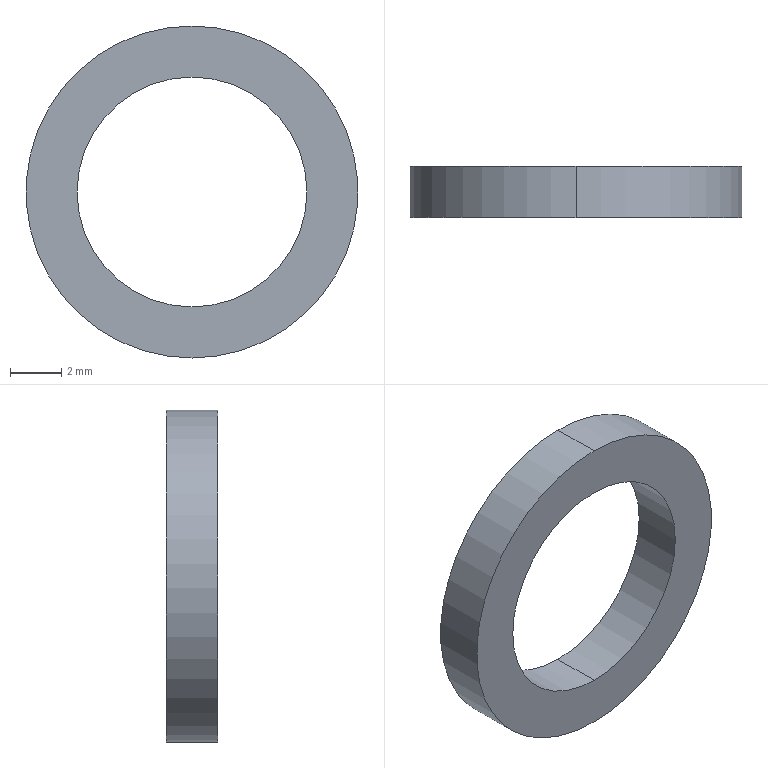Part | NX | features BREP 1 | 1 solid | 6 faces | box 13 x 2 x 13 mm | volume 138.23 mm3 | cylinder 4 | plane 2 | commonest cylinder face diameters 9 x2 13 x2
STEP:
#1=CARTESIAN_POINT('',(0.,2.,-4.5));
#2=VERTEX_POINT('',#1);
#3=CARTESIAN_POINT('',(0.,2.,4.5));
#4=VERTEX_POINT('',#3);
#5=CARTESIAN_POINT('',(0.,2.,0.));
#6=DIRECTION('',(0.,1.,0.));
#7=DIRECTION('',(0.,0.,1.));
#8=AXIS2_PLACEMENT_3D('',#5,#6,#7);
#9=CIRCLE('',#8,4.5);
#10=EDGE_CURVE('',#2,#4,#9,.T.);
#11=ORIENTED_EDGE('',*,*,#10,.T.);
#12=CARTESIAN_POINT('',(0.,0.,4.5));
#13=VERTEX_POINT('',#12);
#14=CARTESIAN_POINT('',(0.,2.,4.5));
#15=DIRECTION('',(0.,-1.,0.));
#16=VECTOR('',#15,1000.);
#17=LINE('',#14,#16);
#18=EDGE_CURVE('',#13,#4,#17,.F.);
#19=ORIENTED_EDGE('',*,*,#18,.F.);
#20=CARTESIAN_POINT('',(0.,0.,-4.5));
#21=VERTEX_POINT('',#20);
#22=CARTESIAN_POINT('',(0.,0.,0.));
#23=DIRECTION('',(0.,1.,0.));
#24=DIRECTION('',(0.,0.,1.));
#25=AXIS2_PLACEMENT_3D('',#22,#23,#24);
#26=CIRCLE('',#25,4.5);
#27=EDGE_CURVE('',#21,#13,#26,.T.);
#28=ORIENTED_EDGE('',*,*,#27,.F.);
#29=CARTESIAN_POINT('',(0.,2.,-4.5));
#30=DIRECTION('',(0.,-1.,0.));
#31=VECTOR('',#30,1000.);
#32=LINE('',#29,#31);
#33=EDGE_CURVE('',#21,#2,#32,.F.);
#34=ORIENTED_EDGE('',*,*,#33,.T.);
#35=EDGE_LOOP('',(#11,#19,#28,#34));
#36=FACE_BOUND('',#35,.T.);
#37=CARTESIAN_POINT('',(0.,2.,0.));
#38=DIRECTION('',(0.,-1.,0.));
#39=DIRECTION('',(0.,0.,1.));
#40=AXIS2_PLACEMENT_3D('',#37,#38,#39);
#41=CYLINDRICAL_SURFACE('',#40,4.5);
#42=ADVANCED_FACE('',(#36),#41,.F.);
#43=CARTESIAN_POINT('',(0.,2.,6.5));
#44=VERTEX_POINT('',#43);
#45=CARTESIAN_POINT('',(0.,2.,-6.5));
#46=VERTEX_POINT('',#45);
#47=CARTESIAN_POINT('',(0.,2.,0.));
#48=DIRECTION('',(0.,1.,0.));
#49=DIRECTION('',(0.,0.,1.));
#50=AXIS2_PLACEMENT_3D('',#47,#48,#49);
#51=CIRCLE('',#50,6.5);
#52=EDGE_CURVE('',#44,#46,#51,.T.);
#53=ORIENTED_EDGE('',*,*,#52,.F.);
#54=CARTESIAN_POINT('',(0.,0.,6.5));
#55=VERTEX_POINT('',#54);
#56=CARTESIAN_POINT('',(0.,2.,6.5));
#57=DIRECTION('',(0.,-1.,0.));
#58=VECTOR('',#57,1000.);
#59=LINE('',#56,#58);
#60=EDGE_CURVE('',#55,#44,#59,.F.);
#61=ORIENTED_EDGE('',*,*,#60,.F.);
#62=CARTESIAN_POINT('',(0.,0.,-6.5));
#63=VERTEX_POINT('',#62);
#64=CARTESIAN_POINT('',(0.,0.,0.));
#65=DIRECTION('',(0.,1.,0.));
#66=DIRECTION('',(0.,0.,1.));
#67=AXIS2_PLACEMENT_3D('',#64,#65,#66);
#68=CIRCLE('',#67,6.5);
#69=EDGE_CURVE('',#55,#63,#68,.T.);
#70=ORIENTED_EDGE('',*,*,#69,.T.);
#71=CARTESIAN_POINT('',(0.,2.,-6.5));
#72=DIRECTION('',(0.,-1.,0.));
#73=VECTOR('',#72,1000.);
#74=LINE('',#71,#73);
#75=EDGE_CURVE('',#63,#46,#74,.F.);
#76=ORIENTED_EDGE('',*,*,#75,.T.);
#77=EDGE_LOOP('',(#53,#61,#70,#76));
#78=FACE_BOUND('',#77,.T.);
#79=CARTESIAN_POINT('',(0.,2.,0.));
#80=DIRECTION('',(0.,-1.,0.));
#81=DIRECTION('',(0.,0.,1.));
#82=AXIS2_PLACEMENT_3D('',#79,#80,#81);
#83=CYLINDRICAL_SURFACE('',#82,6.5);
#84=ADVANCED_FACE('',(#78),#83,.T.);
#85=CARTESIAN_POINT('',(0.,2.,0.));
#86=DIRECTION('',(0.,1.,0.));
#87=DIRECTION('',(0.,0.,1.));
#88=AXIS2_PLACEMENT_3D('',#85,#86,#87);
#89=CIRCLE('',#88,6.5);
#90=EDGE_CURVE('',#46,#44,#89,.T.);
#91=ORIENTED_EDGE('',*,*,#90,.T.);
#92=ORIENTED_EDGE('',*,*,#52,.T.);
#93=EDGE_LOOP('',(#91,#92));
#94=FACE_BOUND('',#93,.T.);
#95=ORIENTED_EDGE('',*,*,#10,.F.);
#96=CARTESIAN_POINT('',(0.,2.,0.));
#97=DIRECTION('',(0.,1.,0.));
#98=DIRECTION('',(0.,0.,1.));
#99=AXIS2_PLACEMENT_3D('',#96,#97,#98);
#100=CIRCLE('',#99,4.5);
#101=EDGE_CURVE('',#4,#2,#100,.T.);
#102=ORIENTED_EDGE('',*,*,#101,.F.);
#103=EDGE_LOOP('',(#95,#102));
#104=FACE_BOUND('',#103,.T.);
#105=CARTESIAN_POINT('',(0.,2.,0.));
#106=DIRECTION('',(0.,1.,0.));
#107=DIRECTION('',(-1.,0.,0.));
#108=AXIS2_PLACEMENT_3D('',#105,#106,#107);
#109=PLANE('',#108);
#110=ADVANCED_FACE('',(#94,#104),#109,.T.);
#111=CARTESIAN_POINT('',(0.,0.,0.));
#112=DIRECTION('',(0.,1.,0.));
#113=DIRECTION('',(0.,0.,1.));
#114=AXIS2_PLACEMENT_3D('',#111,#112,#113);
#115=CIRCLE('',#114,6.5);
#116=EDGE_CURVE('',#63,#55,#115,.T.);
#117=ORIENTED_EDGE('',*,*,#116,.F.);
#118=ORIENTED_EDGE('',*,*,#69,.F.);
#119=EDGE_LOOP('',(#117,#118));
#120=FACE_BOUND('',#119,.T.);
#121=ORIENTED_EDGE('',*,*,#27,.T.);
#122=CARTESIAN_POINT('',(0.,0.,0.));
#123=DIRECTION('',(0.,1.,0.));
#124=DIRECTION('',(0.,0.,1.));
#125=AXIS2_PLACEMENT_3D('',#122,#123,#124);
#126=CIRCLE('',#125,4.5);
#127=EDGE_CURVE('',#13,#21,#126,.T.);
#128=ORIENTED_EDGE('',*,*,#127,.T.);
#129=EDGE_LOOP('',(#121,#128));
#130=FACE_BOUND('',#129,.T.);
#131=CARTESIAN_POINT('',(0.,0.,0.));
#132=DIRECTION('',(0.,1.,0.));
#133=DIRECTION('',(-1.,0.,0.));
#134=AXIS2_PLACEMENT_3D('',#131,#132,#133);
#135=PLANE('',#134);
#136=ADVANCED_FACE('',(#120,#130),#135,.F.);
#137=ORIENTED_EDGE('',*,*,#60,.T.);
#138=ORIENTED_EDGE('',*,*,#90,.F.);
#139=ORIENTED_EDGE('',*,*,#75,.F.);
#140=ORIENTED_EDGE('',*,*,#116,.T.);
#141=EDGE_LOOP('',(#137,#138,#139,#140));
#142=FACE_BOUND('',#141,.T.);
#143=CARTESIAN_POINT('',(0.,2.,0.));
#144=DIRECTION('',(0.,-1.,0.));
#145=DIRECTION('',(0.,0.,1.));
#146=AXIS2_PLACEMENT_3D('',#143,#144,#145);
#147=CYLINDRICAL_SURFACE('',#146,6.5);
#148=ADVANCED_FACE('',(#142),#147,.T.);
#149=ORIENTED_EDGE('',*,*,#18,.T.);
#150=ORIENTED_EDGE('',*,*,#101,.T.);
#151=ORIENTED_EDGE('',*,*,#33,.F.);
#152=ORIENTED_EDGE('',*,*,#127,.F.);
#153=EDGE_LOOP('',(#149,#150,#151,#152));
#154=FACE_BOUND('',#153,.T.);
#155=CARTESIAN_POINT('',(0.,2.,0.));
#156=DIRECTION('',(0.,-1.,0.));
#157=DIRECTION('',(0.,0.,1.));
#158=AXIS2_PLACEMENT_3D('',#155,#156,#157);
#159=CYLINDRICAL_SURFACE('',#158,4.5);
#160=ADVANCED_FACE('',(#154),#159,.F.);
#161=CLOSED_SHELL('',(#42,#84,#110,#136,#148,#160));
#162=MANIFOLD_SOLID_BREP('',#161);
#163=(LENGTH_UNIT()NAMED_UNIT(*)SI_UNIT(.MILLI.,.METRE.));
#164=UNCERTAINTY_MEASURE_WITH_UNIT(LENGTH_MEASURE(0.00001),#163,'','');
#165=(NAMED_UNIT(*)PLANE_ANGLE_UNIT()SI_UNIT($,.RADIAN.));
#166=(NAMED_UNIT(*)SI_UNIT($,.STERADIAN.)SOLID_ANGLE_UNIT());
#167=(GEOMETRIC_REPRESENTATION_CONTEXT(3)GLOBAL_UNCERTAINTY_ASSIGNED_CONTEXT((#164))GLOBAL_UNIT_ASSIGNED_CONTEXT((#163,#165,#166))REPRESENTATION_CONTEXT('',''));
#168=ADVANCED_BREP_SHAPE_REPRESENTATION('',(#162),#167);